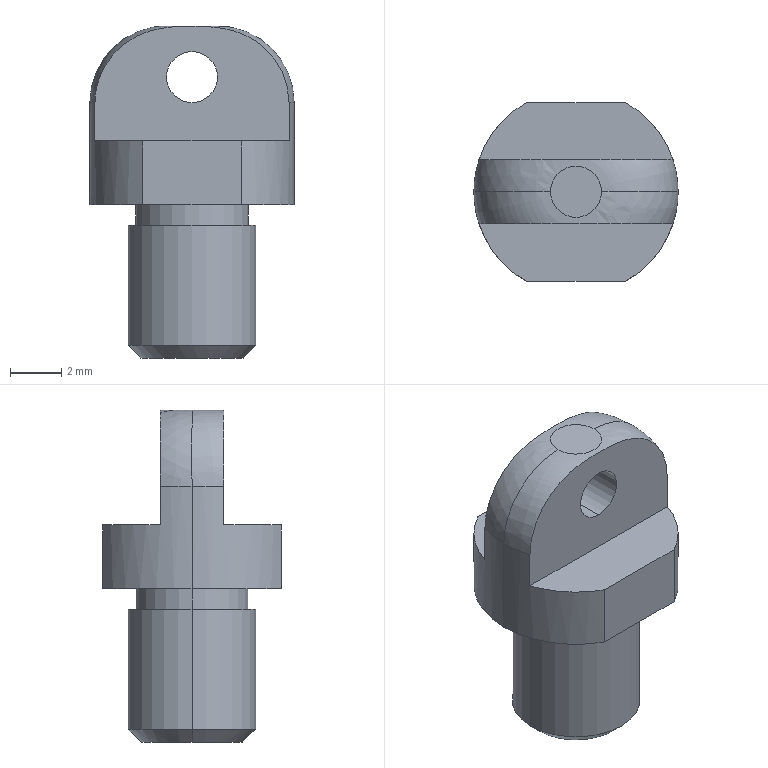Part | STEP file | PN_0025 | 1 solid | 23 faces | box 8 x 7 x 13 mm | volume 302.267 mm3 | plane 10 | cylinder 9 | cone 2 | other 2 | commonest cylinder face diameters 8 x3 2 x2 4.4 x2 5 x2